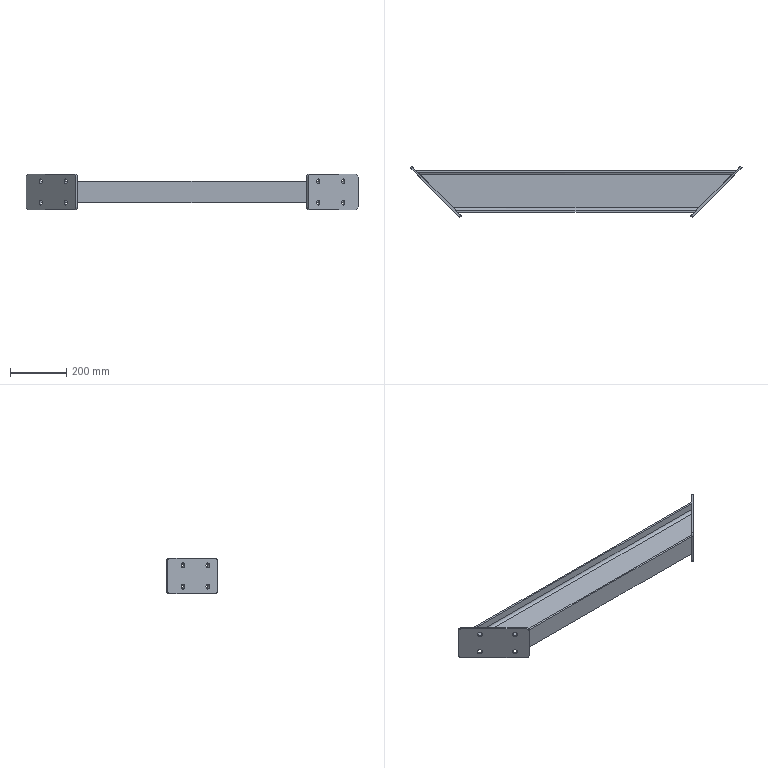Part | STEP file | PN_0060 steel beam brace 1140_Default<As Machined> | 3 solids | 46 faces | box 1178 x 182.434 x 125 mm | volume 2280023 mm3 | plane 26 | cylinder 20 | commonest cylinder face diameters 20 x12 18 x8